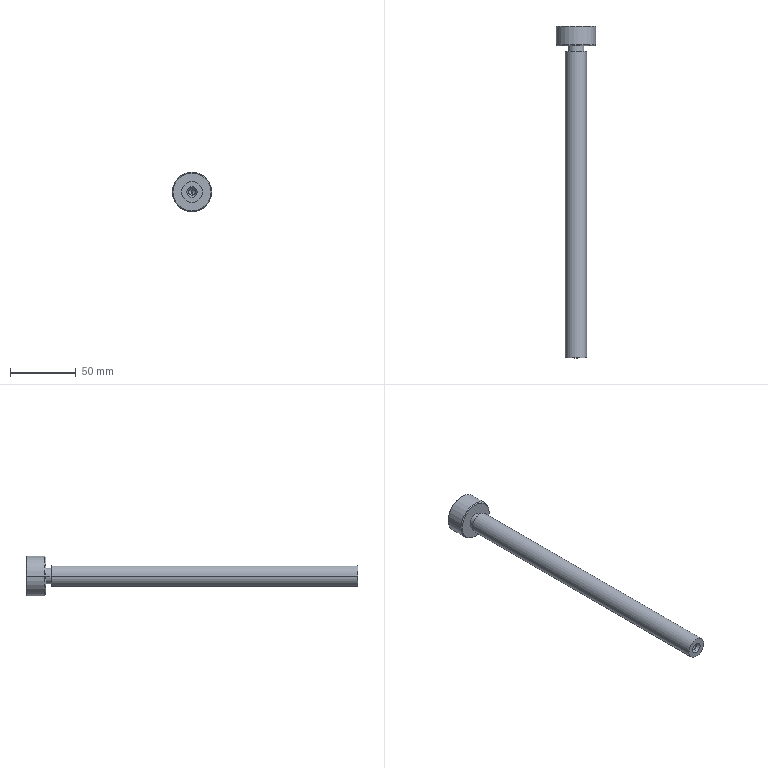Part | SolidWorks | features Chamfer 3, HoleWzd 2, Revolution 1 | 1 solid | 28 faces | box 30 x 252 x 30 mm | volume 57567 mm3 | cone 14 | cylinder 10 | plane 4 | commonest cylinder face diameters 5 x4 12 x2 16 x2 30 x2
STEP:
#1=CARTESIAN_POINT('',(0.,249.504,-2.5));
#2=VERTEX_POINT('',#1);
#3=CARTESIAN_POINT('',(0.,249.504,2.5));
#4=VERTEX_POINT('',#3);
#5=CARTESIAN_POINT('',(0.,249.504,0.));
#6=DIRECTION('',(0.,1.,0.));
#7=DIRECTION('',(0.,0.,-1.));
#8=AXIS2_PLACEMENT_3D('',#5,#6,#7);
#9=CIRCLE('',#8,2.5);
#10=EDGE_CURVE('',#2,#4,#9,.T.);
#11=ORIENTED_EDGE('',*,*,#10,.F.);
#12=CARTESIAN_POINT('',(0.,252.,-4.));
#13=VERTEX_POINT('',#12);
#14=CARTESIAN_POINT('',(0.,249.504,-2.5));
#15=DIRECTION('',(0.,0.8572,-0.515));
#16=VECTOR('',#15,1000.);
#17=LINE('',#14,#16);
#18=EDGE_CURVE('',#2,#13,#17,.T.);
#19=ORIENTED_EDGE('',*,*,#18,.T.);
#20=CARTESIAN_POINT('',(0.,252.,4.));
#21=VERTEX_POINT('',#20);
#22=CARTESIAN_POINT('',(0.,252.,0.));
#23=DIRECTION('',(0.,-1.,0.));
#24=DIRECTION('',(1.,0.,0.));
#25=AXIS2_PLACEMENT_3D('',#22,#23,#24);
#26=CIRCLE('',#25,4.);
#27=EDGE_CURVE('',#21,#13,#26,.T.);
#28=ORIENTED_EDGE('',*,*,#27,.F.);
#29=CARTESIAN_POINT('',(0.,249.504,2.5));
#30=DIRECTION('',(0.,0.8572,0.515));
#31=VECTOR('',#30,1000.);
#32=LINE('',#29,#31);
#33=EDGE_CURVE('',#4,#21,#32,.T.);
#34=ORIENTED_EDGE('',*,*,#33,.F.);
#35=EDGE_LOOP('',(#11,#19,#28,#34));
#36=FACE_OUTER_BOUND('',#35,.T.);
#37=CARTESIAN_POINT('',(0.,249.504,0.));
#38=DIRECTION('',(0.,1.,0.));
#39=DIRECTION('',(0.,0.,1.));
#40=AXIS2_PLACEMENT_3D('',#37,#38,#39);
#41=CONICAL_SURFACE('',#40,2.5,0.5411);
#42=ADVANCED_FACE('',(#36),#41,.F.);
#43=CARTESIAN_POINT('',(0.,247.,-2.5));
#44=VERTEX_POINT('',#43);
#45=CARTESIAN_POINT('',(0.,247.,2.5));
#46=VERTEX_POINT('',#45);
#47=CARTESIAN_POINT('',(0.,247.,0.));
#48=DIRECTION('',(0.,1.,0.));
#49=DIRECTION('',(0.,0.,1.));
#50=AXIS2_PLACEMENT_3D('',#47,#48,#49);
#51=CIRCLE('',#50,2.5);
#52=EDGE_CURVE('',#44,#46,#51,.T.);
#53=ORIENTED_EDGE('',*,*,#52,.F.);
#54=CARTESIAN_POINT('',(0.,252.,-2.5));
#55=DIRECTION('',(0.,1.,0.));
#56=VECTOR('',#55,1000.);
#57=LINE('',#54,#56);
#58=EDGE_CURVE('',#44,#2,#57,.T.);
#59=ORIENTED_EDGE('',*,*,#58,.T.);
#60=ORIENTED_EDGE('',*,*,#10,.T.);
#61=CARTESIAN_POINT('',(0.,252.,2.5));
#62=DIRECTION('',(0.,1.,0.));
#63=VECTOR('',#62,1000.);
#64=LINE('',#61,#63);
#65=EDGE_CURVE('',#46,#4,#64,.T.);
#66=ORIENTED_EDGE('',*,*,#65,.F.);
#67=EDGE_LOOP('',(#53,#59,#60,#66));
#68=FACE_OUTER_BOUND('',#67,.T.);
#69=CARTESIAN_POINT('',(0.,252.,0.));
#70=DIRECTION('',(0.,1.,0.));
#71=DIRECTION('',(0.,0.,1.));
#72=AXIS2_PLACEMENT_3D('',#69,#70,#71);
#73=CYLINDRICAL_SURFACE('',#72,2.5);
#74=ADVANCED_FACE('',(#68),#73,.F.);
#75=CARTESIAN_POINT('',(0.,245.498,0.));
#76=VERTEX_POINT('',#75);
#77=CARTESIAN_POINT('',(0.,247.,2.5));
#78=DIRECTION('',(0.,0.515,0.8572));
#79=VECTOR('',#78,1000.);
#80=LINE('',#77,#79);
#81=EDGE_CURVE('',#76,#46,#80,.T.);
#82=ORIENTED_EDGE('',*,*,#81,.F.);
#83=CARTESIAN_POINT('',(0.,247.,-2.5));
#84=DIRECTION('',(0.,0.515,-0.8572));
#85=VECTOR('',#84,1000.);
#86=LINE('',#83,#85);
#87=EDGE_CURVE('',#76,#44,#86,.T.);
#88=ORIENTED_EDGE('',*,*,#87,.T.);
#89=ORIENTED_EDGE('',*,*,#52,.T.);
#90=EDGE_LOOP('',(#82,#88,#89));
#91=FACE_OUTER_BOUND('',#90,.T.);
#92=CARTESIAN_POINT('',(0.,247.,0.));
#93=DIRECTION('',(0.,1.,0.));
#94=DIRECTION('',(0.,0.,1.));
#95=AXIS2_PLACEMENT_3D('',#92,#93,#94);
#96=CONICAL_SURFACE('',#95,2.5,1.03);
#97=ADVANCED_FACE('',(#91),#96,.F.);
#98=CARTESIAN_POINT('',(-14.168,252.,0.));
#99=VERTEX_POINT('',#98);
#100=CARTESIAN_POINT('',(14.168,252.,0.));
#101=VERTEX_POINT('',#100);
#102=CARTESIAN_POINT('',(0.,252.,0.));
#103=DIRECTION('',(0.,1.,0.));
#104=DIRECTION('',(1.,0.,0.));
#105=AXIS2_PLACEMENT_3D('',#102,#103,#104);
#106=CIRCLE('',#105,14.168);
#107=EDGE_CURVE('',#99,#101,#106,.T.);
#108=ORIENTED_EDGE('',*,*,#107,.F.);
#109=CARTESIAN_POINT('',(-15.,251.5,0.));
#110=VERTEX_POINT('',#109);
#111=CARTESIAN_POINT('',(-14.168,252.,0.));
#112=DIRECTION('',(-0.8572,-0.515,0.));
#113=VECTOR('',#112,1000.);
#114=LINE('',#111,#113);
#115=EDGE_CURVE('',#99,#110,#114,.T.);
#116=ORIENTED_EDGE('',*,*,#115,.T.);
#117=CARTESIAN_POINT('',(15.,251.5,0.));
#118=VERTEX_POINT('',#117);
#119=CARTESIAN_POINT('',(0.,251.5,0.));
#120=DIRECTION('',(0.,-1.,0.));
#121=DIRECTION('',(1.,0.,0.));
#122=AXIS2_PLACEMENT_3D('',#119,#120,#121);
#123=CIRCLE('',#122,15.);
#124=EDGE_CURVE('',#118,#110,#123,.T.);
#125=ORIENTED_EDGE('',*,*,#124,.F.);
#126=CARTESIAN_POINT('',(14.168,252.,0.));
#127=DIRECTION('',(0.8572,-0.515,0.));
#128=VECTOR('',#127,1000.);
#129=LINE('',#126,#128);
#130=EDGE_CURVE('',#101,#118,#129,.T.);
#131=ORIENTED_EDGE('',*,*,#130,.F.);
#132=EDGE_LOOP('',(#108,#116,#125,#131));
#133=FACE_OUTER_BOUND('',#132,.T.);
#134=CARTESIAN_POINT('',(0.,252.,0.));
#135=DIRECTION('',(0.,-1.,0.));
#136=DIRECTION('',(1.,0.,0.));
#137=AXIS2_PLACEMENT_3D('',#134,#135,#136);
#138=CONICAL_SURFACE('',#137,14.168,1.03);
#139=ADVANCED_FACE('',(#133),#138,.T.);
#140=CARTESIAN_POINT('',(14.5,237.,0.));
#141=VERTEX_POINT('',#140);
#142=CARTESIAN_POINT('',(-14.5,237.,0.));
#143=VERTEX_POINT('',#142);
#144=CARTESIAN_POINT('',(0.,237.,0.));
#145=DIRECTION('',(0.,-1.,0.));
#146=DIRECTION('',(-1.,0.,0.));
#147=AXIS2_PLACEMENT_3D('',#144,#145,#146);
#148=CIRCLE('',#147,14.5);
#149=EDGE_CURVE('',#141,#143,#148,.T.);
#150=ORIENTED_EDGE('',*,*,#149,.F.);
#151=CARTESIAN_POINT('',(15.,237.832,0.));
#152=VERTEX_POINT('',#151);
#153=CARTESIAN_POINT('',(15.,237.832,0.));
#154=DIRECTION('',(0.515,0.8572,0.));
#155=VECTOR('',#154,1000.);
#156=LINE('',#153,#155);
#157=EDGE_CURVE('',#141,#152,#156,.T.);
#158=ORIENTED_EDGE('',*,*,#157,.T.);
#159=CARTESIAN_POINT('',(-15.,237.832,0.));
#160=VERTEX_POINT('',#159);
#161=CARTESIAN_POINT('',(0.,237.832,0.));
#162=DIRECTION('',(0.,1.,0.));
#163=DIRECTION('',(-1.,0.,0.));
#164=AXIS2_PLACEMENT_3D('',#161,#162,#163);
#165=CIRCLE('',#164,15.);
#166=EDGE_CURVE('',#160,#152,#165,.T.);
#167=ORIENTED_EDGE('',*,*,#166,.F.);
#168=CARTESIAN_POINT('',(-15.,237.832,0.));
#169=DIRECTION('',(-0.515,0.8572,0.));
#170=VECTOR('',#169,1000.);
#171=LINE('',#168,#170);
#172=EDGE_CURVE('',#143,#160,#171,.T.);
#173=ORIENTED_EDGE('',*,*,#172,.F.);
#174=EDGE_LOOP('',(#150,#158,#167,#173));
#175=FACE_OUTER_BOUND('',#174,.T.);
#176=CARTESIAN_POINT('',(0.,237.832,0.));
#177=DIRECTION('',(0.,1.,0.));
#178=DIRECTION('',(-1.,0.,0.));
#179=AXIS2_PLACEMENT_3D('',#176,#177,#178);
#180=CONICAL_SURFACE('',#179,15.,0.5411);
#181=ADVANCED_FACE('',(#175),#180,.T.);
#182=CARTESIAN_POINT('',(-7.168,233.,0.));
#183=VERTEX_POINT('',#182);
#184=CARTESIAN_POINT('',(7.168,233.,0.));
#185=VERTEX_POINT('',#184);
#186=CARTESIAN_POINT('',(0.,233.,0.));
#187=DIRECTION('',(0.,1.,0.));
#188=DIRECTION('',(1.,0.,0.));
#189=AXIS2_PLACEMENT_3D('',#186,#187,#188);
#190=CIRCLE('',#189,7.168);
#191=EDGE_CURVE('',#183,#185,#190,.T.);
#192=ORIENTED_EDGE('',*,*,#191,.F.);
#193=CARTESIAN_POINT('',(-8.,232.5,0.));
#194=VERTEX_POINT('',#193);
#195=CARTESIAN_POINT('',(-7.168,233.,0.));
#196=DIRECTION('',(-0.8572,-0.515,0.));
#197=VECTOR('',#196,1000.);
#198=LINE('',#195,#197);
#199=EDGE_CURVE('',#183,#194,#198,.T.);
#200=ORIENTED_EDGE('',*,*,#199,.T.);
#201=CARTESIAN_POINT('',(8.,232.5,0.));
#202=VERTEX_POINT('',#201);
#203=CARTESIAN_POINT('',(0.,232.5,0.));
#204=DIRECTION('',(0.,-1.,0.));
#205=DIRECTION('',(1.,0.,0.));
#206=AXIS2_PLACEMENT_3D('',#203,#204,#205);
#207=CIRCLE('',#206,8.);
#208=EDGE_CURVE('',#202,#194,#207,.T.);
#209=ORIENTED_EDGE('',*,*,#208,.F.);
#210=CARTESIAN_POINT('',(7.168,233.,0.));
#211=DIRECTION('',(0.8572,-0.515,0.));
#212=VECTOR('',#211,1000.);
#213=LINE('',#210,#212);
#214=EDGE_CURVE('',#185,#202,#213,.T.);
#215=ORIENTED_EDGE('',*,*,#214,.F.);
#216=EDGE_LOOP('',(#192,#200,#209,#215));
#217=FACE_OUTER_BOUND('',#216,.T.);
#218=CARTESIAN_POINT('',(0.,233.,0.));
#219=DIRECTION('',(0.,-1.,0.));
#220=DIRECTION('',(1.,0.,0.));
#221=AXIS2_PLACEMENT_3D('',#218,#219,#220);
#222=CONICAL_SURFACE('',#221,7.168,1.03);
#223=ADVANCED_FACE('',(#217),#222,.T.);
#224=CARTESIAN_POINT('',(0.,2.496,2.5));
#225=VERTEX_POINT('',#224);
#226=CARTESIAN_POINT('',(0.,2.496,-2.5));
#227=VERTEX_POINT('',#226);
#228=CARTESIAN_POINT('',(0.,2.496,0.));
#229=DIRECTION('',(0.,-1.,0.));
#230=DIRECTION('',(0.,0.,1.));
#231=AXIS2_PLACEMENT_3D('',#228,#229,#230);
#232=CIRCLE('',#231,2.5);
#233=EDGE_CURVE('',#225,#227,#232,.T.);
#234=ORIENTED_EDGE('',*,*,#233,.F.);
#235=CARTESIAN_POINT('',(0.,0.,4.));
#236=VERTEX_POINT('',#235);
#237=CARTESIAN_POINT('',(0.,2.496,2.5));
#238=DIRECTION('',(0.,-0.8572,0.515));
#239=VECTOR('',#238,1000.);
#240=LINE('',#237,#239);
#241=EDGE_CURVE('',#225,#236,#240,.T.);
#242=ORIENTED_EDGE('',*,*,#241,.T.);
#243=CARTESIAN_POINT('',(0.,0.,-4.));
#244=VERTEX_POINT('',#243);
#245=CARTESIAN_POINT('',(0.,0.,0.));
#246=DIRECTION('',(0.,1.,0.));
#247=DIRECTION('',(-1.,0.,0.));
#248=AXIS2_PLACEMENT_3D('',#245,#246,#247);
#249=CIRCLE('',#248,4.);
#250=EDGE_CURVE('',#244,#236,#249,.T.);
#251=ORIENTED_EDGE('',*,*,#250,.F.);
#252=CARTESIAN_POINT('',(0.,2.496,-2.5));
#253=DIRECTION('',(0.,-0.8572,-0.515));
#254=VECTOR('',#253,1000.);
#255=LINE('',#252,#254);
#256=EDGE_CURVE('',#227,#244,#255,.T.);
#257=ORIENTED_EDGE('',*,*,#256,.F.);
#258=EDGE_LOOP('',(#234,#242,#251,#257));
#259=FACE_OUTER_BOUND('',#258,.T.);
#260=CARTESIAN_POINT('',(0.,2.496,0.));
#261=DIRECTION('',(0.,-1.,0.));
#262=DIRECTION('',(0.,0.,-1.));
#263=AXIS2_PLACEMENT_3D('',#260,#261,#262);
#264=CONICAL_SURFACE('',#263,2.5,0.5411);
#265=ADVANCED_FACE('',(#259),#264,.F.);
#266=CARTESIAN_POINT('',(0.,5.,2.5));
#267=VERTEX_POINT('',#266);
#268=CARTESIAN_POINT('',(0.,5.,-2.5));
#269=VERTEX_POINT('',#268);
#270=CARTESIAN_POINT('',(0.,5.,0.));
#271=DIRECTION('',(0.,-1.,0.));
#272=DIRECTION('',(0.,0.,-1.));
#273=AXIS2_PLACEMENT_3D('',#270,#271,#272);
#274=CIRCLE('',#273,2.5);
#275=EDGE_CURVE('',#267,#269,#274,.T.);
#276=ORIENTED_EDGE('',*,*,#275,.F.);
#277=CARTESIAN_POINT('',(0.,0.,2.5));
#278=DIRECTION('',(0.,-1.,0.));
#279=VECTOR('',#278,1000.);
#280=LINE('',#277,#279);
#281=EDGE_CURVE('',#267,#225,#280,.T.);
#282=ORIENTED_EDGE('',*,*,#281,.T.);
#283=ORIENTED_EDGE('',*,*,#233,.T.);
#284=CARTESIAN_POINT('',(0.,0.,-2.5));
#285=DIRECTION('',(0.,-1.,0.));
#286=VECTOR('',#285,1000.);
#287=LINE('',#284,#286);
#288=EDGE_CURVE('',#269,#227,#287,.T.);
#289=ORIENTED_EDGE('',*,*,#288,.F.);
#290=EDGE_LOOP('',(#276,#282,#283,#289));
#291=FACE_OUTER_BOUND('',#290,.T.);
#292=CARTESIAN_POINT('',(0.,0.,0.));
#293=DIRECTION('',(0.,-1.,0.));
#294=DIRECTION('',(0.,0.,-1.));
#295=AXIS2_PLACEMENT_3D('',#292,#293,#294);
#296=CYLINDRICAL_SURFACE('',#295,2.5);
#297=ADVANCED_FACE('',(#291),#296,.F.);
#298=CARTESIAN_POINT('',(0.,6.502,0.));
#299=VERTEX_POINT('',#298);
#300=CARTESIAN_POINT('',(0.,5.,-2.5));
#301=DIRECTION('',(0.,-0.515,-0.8572));
#302=VECTOR('',#301,1000.);
#303=LINE('',#300,#302);
#304=EDGE_CURVE('',#299,#269,#303,.T.);
#305=ORIENTED_EDGE('',*,*,#304,.F.);
#306=CARTESIAN_POINT('',(0.,5.,2.5));
#307=DIRECTION('',(0.,-0.515,0.8572));
#308=VECTOR('',#307,1000.);
#309=LINE('',#306,#308);
#310=EDGE_CURVE('',#299,#267,#309,.T.);
#311=ORIENTED_EDGE('',*,*,#310,.T.);
#312=ORIENTED_EDGE('',*,*,#275,.T.);
#313=EDGE_LOOP('',(#305,#311,#312));
#314=FACE_OUTER_BOUND('',#313,.T.);
#315=CARTESIAN_POINT('',(0.,5.,0.));
#316=DIRECTION('',(0.,-1.,0.));
#317=DIRECTION('',(0.,0.,-1.));
#318=AXIS2_PLACEMENT_3D('',#315,#316,#317);
#319=CONICAL_SURFACE('',#318,2.5,1.03);
#320=ADVANCED_FACE('',(#314),#319,.F.);
#321=ORIENTED_EDGE('',*,*,#166,.T.);
#322=CARTESIAN_POINT('',(15.,252.,0.));
#323=DIRECTION('',(0.,1.,0.));
#324=VECTOR('',#323,1000.);
#325=LINE('',#322,#324);
#326=EDGE_CURVE('',#152,#118,#325,.T.);
#327=ORIENTED_EDGE('',*,*,#326,.T.);
#328=ORIENTED_EDGE('',*,*,#124,.T.);
#329=CARTESIAN_POINT('',(-15.,252.,0.));
#330=DIRECTION('',(0.,1.,0.));
#331=VECTOR('',#330,1000.);
#332=LINE('',#329,#331);
#333=EDGE_CURVE('',#160,#110,#332,.T.);
#334=ORIENTED_EDGE('',*,*,#333,.F.);
#335=EDGE_LOOP('',(#321,#327,#328,#334));
#336=FACE_OUTER_BOUND('',#335,.T.);
#337=CARTESIAN_POINT('',(0.,252.,0.));
#338=DIRECTION('',(0.,1.,0.));
#339=DIRECTION('',(-1.,0.,0.));
#340=AXIS2_PLACEMENT_3D('',#337,#338,#339);
#341=CYLINDRICAL_SURFACE('',#340,15.);
#342=ADVANCED_FACE('',(#336),#341,.T.);
#343=CARTESIAN_POINT('',(-8.,0.,0.));
#344=VERTEX_POINT('',#343);
#345=CARTESIAN_POINT('',(8.,0.,0.));
#346=VERTEX_POINT('',#345);
#347=CARTESIAN_POINT('',(0.,0.,0.));
#348=DIRECTION('',(0.,1.,0.));
#349=DIRECTION('',(-1.,0.,0.));
#350=AXIS2_PLACEMENT_3D('',#347,#348,#349);
#351=CIRCLE('',#350,8.);
#352=EDGE_CURVE('',#344,#346,#351,.T.);
#353=ORIENTED_EDGE('',*,*,#352,.T.);
#354=CARTESIAN_POINT('',(8.,252.,0.));
#355=DIRECTION('',(0.,1.,0.));
#356=VECTOR('',#355,1000.);
#357=LINE('',#354,#356);
#358=EDGE_CURVE('',#346,#202,#357,.T.);
#359=ORIENTED_EDGE('',*,*,#358,.T.);
#360=ORIENTED_EDGE('',*,*,#208,.T.);
#361=CARTESIAN_POINT('',(-8.,252.,0.));
#362=DIRECTION('',(0.,1.,0.));
#363=VECTOR('',#362,1000.);
#364=LINE('',#361,#363);
#365=EDGE_CURVE('',#344,#194,#364,.T.);
#366=ORIENTED_EDGE('',*,*,#365,.F.);
#367=EDGE_LOOP('',(#353,#359,#360,#366));
#368=FACE_OUTER_BOUND('',#367,.T.);
#369=CARTESIAN_POINT('',(0.,252.,0.));
#370=DIRECTION('',(0.,1.,0.));
#371=DIRECTION('',(-1.,0.,0.));
#372=AXIS2_PLACEMENT_3D('',#369,#370,#371);
#373=CYLINDRICAL_SURFACE('',#372,8.);
#374=ADVANCED_FACE('',(#368),#373,.T.);
#375=CARTESIAN_POINT('',(-6.,233.,0.));
#376=VERTEX_POINT('',#375);
#377=CARTESIAN_POINT('',(6.,233.,0.));
#378=VERTEX_POINT('',#377);
#379=CARTESIAN_POINT('',(0.,233.,0.));
#380=DIRECTION('',(0.,1.,0.));
#381=DIRECTION('',(-1.,0.,0.));
#382=AXIS2_PLACEMENT_3D('',#379,#380,#381);
#383=CIRCLE('',#382,6.);
#384=EDGE_CURVE('',#376,#378,#383,.T.);
#385=ORIENTED_EDGE('',*,*,#384,.T.);
#386=CARTESIAN_POINT('',(6.,237.,0.));
#387=VERTEX_POINT('',#386);
#388=CARTESIAN_POINT('',(6.,252.,0.));
#389=DIRECTION('',(0.,1.,0.));
#390=VECTOR('',#389,1000.);
#391=LINE('',#388,#390);
#392=EDGE_CURVE('',#378,#387,#391,.T.);
#393=ORIENTED_EDGE('',*,*,#392,.T.);
#394=CARTESIAN_POINT('',(-6.,237.,0.));
#395=VERTEX_POINT('',#394);
#396=CARTESIAN_POINT('',(0.,237.,0.));
#397=DIRECTION('',(0.,1.,0.));
#398=DIRECTION('',(-1.,0.,0.));
#399=AXIS2_PLACEMENT_3D('',#396,#397,#398);
#400=CIRCLE('',#399,6.);
#401=EDGE_CURVE('',#395,#387,#400,.T.);
#402=ORIENTED_EDGE('',*,*,#401,.F.);
#403=CARTESIAN_POINT('',(-6.,252.,0.));
#404=DIRECTION('',(0.,1.,0.));
#405=VECTOR('',#404,1000.);
#406=LINE('',#403,#405);
#407=EDGE_CURVE('',#376,#395,#406,.T.);
#408=ORIENTED_EDGE('',*,*,#407,.F.);
#409=EDGE_LOOP('',(#385,#393,#402,#408));
#410=FACE_OUTER_BOUND('',#409,.T.);
#411=CARTESIAN_POINT('',(0.,252.,0.));
#412=DIRECTION('',(0.,1.,0.));
#413=DIRECTION('',(-1.,0.,0.));
#414=AXIS2_PLACEMENT_3D('',#411,#412,#413);
#415=CYLINDRICAL_SURFACE('',#414,6.);
#416=ADVANCED_FACE('',(#410),#415,.T.);
#417=ORIENTED_EDGE('',*,*,#392,.F.);
#418=CARTESIAN_POINT('',(0.,233.,0.));
#419=DIRECTION('',(0.,1.,0.));
#420=DIRECTION('',(-1.,0.,0.));
#421=AXIS2_PLACEMENT_3D('',#418,#419,#420);
#422=CIRCLE('',#421,6.);
#423=EDGE_CURVE('',#378,#376,#422,.T.);
#424=ORIENTED_EDGE('',*,*,#423,.T.);
#425=ORIENTED_EDGE('',*,*,#407,.T.);
#426=CARTESIAN_POINT('',(0.,237.,0.));
#427=DIRECTION('',(0.,1.,0.));
#428=DIRECTION('',(-1.,0.,0.));
#429=AXIS2_PLACEMENT_3D('',#426,#427,#428);
#430=CIRCLE('',#429,6.);
#431=EDGE_CURVE('',#387,#395,#430,.T.);
#432=ORIENTED_EDGE('',*,*,#431,.F.);
#433=EDGE_LOOP('',(#417,#424,#425,#432));
#434=FACE_OUTER_BOUND('',#433,.T.);
#435=CARTESIAN_POINT('',(0.,252.,0.));
#436=DIRECTION('',(0.,1.,0.));
#437=DIRECTION('',(-1.,0.,0.));
#438=AXIS2_PLACEMENT_3D('',#435,#436,#437);
#439=CYLINDRICAL_SURFACE('',#438,6.);
#440=ADVANCED_FACE('',(#434),#439,.T.);
#441=CARTESIAN_POINT('',(0.,233.,0.));
#442=DIRECTION('',(0.,1.,0.));
#443=DIRECTION('',(1.,0.,0.));
#444=AXIS2_PLACEMENT_3D('',#441,#442,#443);
#445=CIRCLE('',#444,7.168);
#446=EDGE_CURVE('',#185,#183,#445,.T.);
#447=ORIENTED_EDGE('',*,*,#446,.T.);
#448=ORIENTED_EDGE('',*,*,#191,.T.);
#449=EDGE_LOOP('',(#447,#448));
#450=FACE_OUTER_BOUND('',#449,.T.);
#451=ORIENTED_EDGE('',*,*,#384,.F.);
#452=ORIENTED_EDGE('',*,*,#423,.F.);
#453=EDGE_LOOP('',(#451,#452));
#454=FACE_BOUND('',#453,.T.);
#455=CARTESIAN_POINT('',(8.,233.,0.));
#456=DIRECTION('',(0.,-1.,0.));
#457=DIRECTION('',(1.,0.,0.));
#458=AXIS2_PLACEMENT_3D('',#455,#456,#457);
#459=PLANE('',#458);
#460=ADVANCED_FACE('',(#450,#454),#459,.F.);
#461=ORIENTED_EDGE('',*,*,#358,.F.);
#462=CARTESIAN_POINT('',(0.,0.,0.));
#463=DIRECTION('',(0.,1.,0.));
#464=DIRECTION('',(-1.,0.,0.));
#465=AXIS2_PLACEMENT_3D('',#462,#463,#464);
#466=CIRCLE('',#465,8.);
#467=EDGE_CURVE('',#346,#344,#466,.T.);
#468=ORIENTED_EDGE('',*,*,#467,.T.);
#469=ORIENTED_EDGE('',*,*,#365,.T.);
#470=CARTESIAN_POINT('',(0.,232.5,0.));
#471=DIRECTION('',(0.,-1.,0.));
#472=DIRECTION('',(1.,0.,0.));
#473=AXIS2_PLACEMENT_3D('',#470,#471,#472);
#474=CIRCLE('',#473,8.);
#475=EDGE_CURVE('',#194,#202,#474,.T.);
#476=ORIENTED_EDGE('',*,*,#475,.T.);
#477=EDGE_LOOP('',(#461,#468,#469,#476));
#478=FACE_OUTER_BOUND('',#477,.T.);
#479=CARTESIAN_POINT('',(0.,252.,0.));
#480=DIRECTION('',(0.,1.,0.));
#481=DIRECTION('',(-1.,0.,0.));
#482=AXIS2_PLACEMENT_3D('',#479,#480,#481);
#483=CYLINDRICAL_SURFACE('',#482,8.);
#484=ADVANCED_FACE('',(#478),#483,.T.);
#485=ORIENTED_EDGE('',*,*,#250,.T.);
#486=CARTESIAN_POINT('',(0.,0.,0.));
#487=DIRECTION('',(0.,1.,0.));
#488=DIRECTION('',(-1.,0.,0.));
#489=AXIS2_PLACEMENT_3D('',#486,#487,#488);
#490=CIRCLE('',#489,4.);
#491=EDGE_CURVE('',#236,#244,#490,.T.);
#492=ORIENTED_EDGE('',*,*,#491,.T.);
#493=EDGE_LOOP('',(#485,#492));
#494=FACE_BOUND('',#493,.T.);
#495=ORIENTED_EDGE('',*,*,#352,.F.);
#496=ORIENTED_EDGE('',*,*,#467,.F.);
#497=EDGE_LOOP('',(#495,#496));
#498=FACE_OUTER_BOUND('',#497,.T.);
#499=CARTESIAN_POINT('',(0.,0.,0.));
#500=DIRECTION('',(0.,1.,0.));
#501=DIRECTION('',(-1.,0.,0.));
#502=AXIS2_PLACEMENT_3D('',#499,#500,#501);
#503=PLANE('',#502);
#504=ADVANCED_FACE('',(#494,#498),#503,.F.);
#505=ORIENTED_EDGE('',*,*,#27,.T.);
#506=CARTESIAN_POINT('',(0.,252.,0.));
#507=DIRECTION('',(0.,-1.,0.));
#508=DIRECTION('',(1.,0.,0.));
#509=AXIS2_PLACEMENT_3D('',#506,#507,#508);
#510=CIRCLE('',#509,4.);
#511=EDGE_CURVE('',#13,#21,#510,.T.);
#512=ORIENTED_EDGE('',*,*,#511,.T.);
#513=EDGE_LOOP('',(#505,#512));
#514=FACE_BOUND('',#513,.T.);
#515=CARTESIAN_POINT('',(0.,252.,0.));
#516=DIRECTION('',(0.,1.,0.));
#517=DIRECTION('',(1.,0.,0.));
#518=AXIS2_PLACEMENT_3D('',#515,#516,#517);
#519=CIRCLE('',#518,14.168);
#520=EDGE_CURVE('',#101,#99,#519,.T.);
#521=ORIENTED_EDGE('',*,*,#520,.T.);
#522=ORIENTED_EDGE('',*,*,#107,.T.);
#523=EDGE_LOOP('',(#521,#522));
#524=FACE_OUTER_BOUND('',#523,.T.);
#525=CARTESIAN_POINT('',(0.,252.,0.));
#526=DIRECTION('',(0.,-1.,0.));
#527=DIRECTION('',(1.,0.,0.));
#528=AXIS2_PLACEMENT_3D('',#525,#526,#527);
#529=PLANE('',#528);
#530=ADVANCED_FACE('',(#514,#524),#529,.F.);
#531=ORIENTED_EDGE('',*,*,#326,.F.);
#532=CARTESIAN_POINT('',(0.,237.832,0.));
#533=DIRECTION('',(0.,1.,0.));
#534=DIRECTION('',(-1.,0.,0.));
#535=AXIS2_PLACEMENT_3D('',#532,#533,#534);
#536=CIRCLE('',#535,15.);
#537=EDGE_CURVE('',#152,#160,#536,.T.);
#538=ORIENTED_EDGE('',*,*,#537,.T.);
#539=ORIENTED_EDGE('',*,*,#333,.T.);
#540=CARTESIAN_POINT('',(0.,251.5,0.));
#541=DIRECTION('',(0.,-1.,0.));
#542=DIRECTION('',(1.,0.,0.));
#543=AXIS2_PLACEMENT_3D('',#540,#541,#542);
#544=CIRCLE('',#543,15.);
#545=EDGE_CURVE('',#110,#118,#544,.T.);
#546=ORIENTED_EDGE('',*,*,#545,.T.);
#547=EDGE_LOOP('',(#531,#538,#539,#546));
#548=FACE_OUTER_BOUND('',#547,.T.);
#549=CARTESIAN_POINT('',(0.,252.,0.));
#550=DIRECTION('',(0.,1.,0.));
#551=DIRECTION('',(-1.,0.,0.));
#552=AXIS2_PLACEMENT_3D('',#549,#550,#551);
#553=CYLINDRICAL_SURFACE('',#552,15.);
#554=ADVANCED_FACE('',(#548),#553,.T.);
#555=CARTESIAN_POINT('',(0.,237.,0.));
#556=DIRECTION('',(0.,-1.,0.));
#557=DIRECTION('',(-1.,0.,0.));
#558=AXIS2_PLACEMENT_3D('',#555,#556,#557);
#559=CIRCLE('',#558,14.5);
#560=EDGE_CURVE('',#143,#141,#559,.T.);
#561=ORIENTED_EDGE('',*,*,#560,.T.);
#562=ORIENTED_EDGE('',*,*,#149,.T.);
#563=EDGE_LOOP('',(#561,#562));
#564=FACE_OUTER_BOUND('',#563,.T.);
#565=ORIENTED_EDGE('',*,*,#401,.T.);
#566=ORIENTED_EDGE('',*,*,#431,.T.);
#567=EDGE_LOOP('',(#565,#566));
#568=FACE_BOUND('',#567,.T.);
#569=CARTESIAN_POINT('',(15.,237.,0.));
#570=DIRECTION('',(0.,1.,0.));
#571=DIRECTION('',(-1.,0.,0.));
#572=AXIS2_PLACEMENT_3D('',#569,#570,#571);
#573=PLANE('',#572);
#574=ADVANCED_FACE('',(#564,#568),#573,.F.);
#575=ORIENTED_EDGE('',*,*,#310,.F.);
#576=ORIENTED_EDGE('',*,*,#304,.T.);
#577=CARTESIAN_POINT('',(0.,5.,0.));
#578=DIRECTION('',(0.,-1.,0.));
#579=DIRECTION('',(0.,0.,-1.));
#580=AXIS2_PLACEMENT_3D('',#577,#578,#579);
#581=CIRCLE('',#580,2.5);
#582=EDGE_CURVE('',#269,#267,#581,.T.);
#583=ORIENTED_EDGE('',*,*,#582,.T.);
#584=EDGE_LOOP('',(#575,#576,#583));
#585=FACE_OUTER_BOUND('',#584,.T.);
#586=CARTESIAN_POINT('',(0.,5.,0.));
#587=DIRECTION('',(0.,-1.,0.));
#588=DIRECTION('',(0.,0.,-1.));
#589=AXIS2_PLACEMENT_3D('',#586,#587,#588);
#590=CONICAL_SURFACE('',#589,2.5,1.03);
#591=ADVANCED_FACE('',(#585),#590,.F.);
#592=ORIENTED_EDGE('',*,*,#281,.F.);
#593=ORIENTED_EDGE('',*,*,#582,.F.);
#594=ORIENTED_EDGE('',*,*,#288,.T.);
#595=CARTESIAN_POINT('',(0.,2.496,0.));
#596=DIRECTION('',(0.,-1.,0.));
#597=DIRECTION('',(0.,0.,1.));
#598=AXIS2_PLACEMENT_3D('',#595,#596,#597);
#599=CIRCLE('',#598,2.5);
#600=EDGE_CURVE('',#227,#225,#599,.T.);
#601=ORIENTED_EDGE('',*,*,#600,.T.);
#602=EDGE_LOOP('',(#592,#593,#594,#601));
#603=FACE_OUTER_BOUND('',#602,.T.);
#604=CARTESIAN_POINT('',(0.,0.,0.));
#605=DIRECTION('',(0.,-1.,0.));
#606=DIRECTION('',(0.,0.,-1.));
#607=AXIS2_PLACEMENT_3D('',#604,#605,#606);
#608=CYLINDRICAL_SURFACE('',#607,2.5);
#609=ADVANCED_FACE('',(#603),#608,.F.);
#610=ORIENTED_EDGE('',*,*,#241,.F.);
#611=ORIENTED_EDGE('',*,*,#600,.F.);
#612=ORIENTED_EDGE('',*,*,#256,.T.);
#613=ORIENTED_EDGE('',*,*,#491,.F.);
#614=EDGE_LOOP('',(#610,#611,#612,#613));
#615=FACE_OUTER_BOUND('',#614,.T.);
#616=CARTESIAN_POINT('',(0.,2.496,0.));
#617=DIRECTION('',(0.,-1.,0.));
#618=DIRECTION('',(0.,0.,-1.));
#619=AXIS2_PLACEMENT_3D('',#616,#617,#618);
#620=CONICAL_SURFACE('',#619,2.5,0.5411);
#621=ADVANCED_FACE('',(#615),#620,.F.);
#622=ORIENTED_EDGE('',*,*,#199,.F.);
#623=ORIENTED_EDGE('',*,*,#446,.F.);
#624=ORIENTED_EDGE('',*,*,#214,.T.);
#625=ORIENTED_EDGE('',*,*,#475,.F.);
#626=EDGE_LOOP('',(#622,#623,#624,#625));
#627=FACE_OUTER_BOUND('',#626,.T.);
#628=CARTESIAN_POINT('',(0.,233.,0.));
#629=DIRECTION('',(0.,-1.,0.));
#630=DIRECTION('',(1.,0.,0.));
#631=AXIS2_PLACEMENT_3D('',#628,#629,#630);
#632=CONICAL_SURFACE('',#631,7.168,1.03);
#633=ADVANCED_FACE('',(#627),#632,.T.);
#634=ORIENTED_EDGE('',*,*,#157,.F.);
#635=ORIENTED_EDGE('',*,*,#560,.F.);
#636=ORIENTED_EDGE('',*,*,#172,.T.);
#637=ORIENTED_EDGE('',*,*,#537,.F.);
#638=EDGE_LOOP('',(#634,#635,#636,#637));
#639=FACE_OUTER_BOUND('',#638,.T.);
#640=CARTESIAN_POINT('',(0.,237.832,0.));
#641=DIRECTION('',(0.,1.,0.));
#642=DIRECTION('',(-1.,0.,0.));
#643=AXIS2_PLACEMENT_3D('',#640,#641,#642);
#644=CONICAL_SURFACE('',#643,15.,0.5411);
#645=ADVANCED_FACE('',(#639),#644,.T.);
#646=ORIENTED_EDGE('',*,*,#115,.F.);
#647=ORIENTED_EDGE('',*,*,#520,.F.);
#648=ORIENTED_EDGE('',*,*,#130,.T.);
#649=ORIENTED_EDGE('',*,*,#545,.F.);
#650=EDGE_LOOP('',(#646,#647,#648,#649));
#651=FACE_OUTER_BOUND('',#650,.T.);
#652=CARTESIAN_POINT('',(0.,252.,0.));
#653=DIRECTION('',(0.,-1.,0.));
#654=DIRECTION('',(1.,0.,0.));
#655=AXIS2_PLACEMENT_3D('',#652,#653,#654);
#656=CONICAL_SURFACE('',#655,14.168,1.03);
#657=ADVANCED_FACE('',(#651),#656,.T.);
#658=ORIENTED_EDGE('',*,*,#87,.F.);
#659=ORIENTED_EDGE('',*,*,#81,.T.);
#660=CARTESIAN_POINT('',(0.,247.,0.));
#661=DIRECTION('',(0.,1.,0.));
#662=DIRECTION('',(0.,0.,1.));
#663=AXIS2_PLACEMENT_3D('',#660,#661,#662);
#664=CIRCLE('',#663,2.5);
#665=EDGE_CURVE('',#46,#44,#664,.T.);
#666=ORIENTED_EDGE('',*,*,#665,.T.);
#667=EDGE_LOOP('',(#658,#659,#666));
#668=FACE_OUTER_BOUND('',#667,.T.);
#669=CARTESIAN_POINT('',(0.,247.,0.));
#670=DIRECTION('',(0.,1.,0.));
#671=DIRECTION('',(0.,0.,1.));
#672=AXIS2_PLACEMENT_3D('',#669,#670,#671);
#673=CONICAL_SURFACE('',#672,2.5,1.03);
#674=ADVANCED_FACE('',(#668),#673,.F.);
#675=ORIENTED_EDGE('',*,*,#58,.F.);
#676=ORIENTED_EDGE('',*,*,#665,.F.);
#677=ORIENTED_EDGE('',*,*,#65,.T.);
#678=CARTESIAN_POINT('',(0.,249.504,0.));
#679=DIRECTION('',(0.,1.,0.));
#680=DIRECTION('',(0.,0.,-1.));
#681=AXIS2_PLACEMENT_3D('',#678,#679,#680);
#682=CIRCLE('',#681,2.5);
#683=EDGE_CURVE('',#4,#2,#682,.T.);
#684=ORIENTED_EDGE('',*,*,#683,.T.);
#685=EDGE_LOOP('',(#675,#676,#677,#684));
#686=FACE_OUTER_BOUND('',#685,.T.);
#687=CARTESIAN_POINT('',(0.,252.,0.));
#688=DIRECTION('',(0.,1.,0.));
#689=DIRECTION('',(0.,0.,1.));
#690=AXIS2_PLACEMENT_3D('',#687,#688,#689);
#691=CYLINDRICAL_SURFACE('',#690,2.5);
#692=ADVANCED_FACE('',(#686),#691,.F.);
#693=ORIENTED_EDGE('',*,*,#18,.F.);
#694=ORIENTED_EDGE('',*,*,#683,.F.);
#695=ORIENTED_EDGE('',*,*,#33,.T.);
#696=ORIENTED_EDGE('',*,*,#511,.F.);
#697=EDGE_LOOP('',(#693,#694,#695,#696));
#698=FACE_OUTER_BOUND('',#697,.T.);
#699=CARTESIAN_POINT('',(0.,249.504,0.));
#700=DIRECTION('',(0.,1.,0.));
#701=DIRECTION('',(0.,0.,1.));
#702=AXIS2_PLACEMENT_3D('',#699,#700,#701);
#703=CONICAL_SURFACE('',#702,2.5,0.5411);
#704=ADVANCED_FACE('',(#698),#703,.F.);
#705=CLOSED_SHELL('',(#42,#74,#97,#139,#181,#223,#265,#297,#320,#342,#374,#416,#440,#460,#484,#504,#530,#554,#574,#591,#609,#621,#633,#645,#657,#674,#692,#704));
#706=MANIFOLD_SOLID_BREP('',#705);
#707=CARTESIAN_POINT('',(0.,0.,0.));
#708=DIRECTION('',(0.,0.,1.));
#709=DIRECTION('',(1.,0.,0.));
#710=AXIS2_PLACEMENT_3D('',#707,#708,#709);
#711=(LENGTH_UNIT()NAMED_UNIT(*)SI_UNIT(.MILLI.,.METRE.));
#712=UNCERTAINTY_MEASURE_WITH_UNIT(LENGTH_MEASURE(0.00001),#711,'','');
#713=(NAMED_UNIT(*)PLANE_ANGLE_UNIT()SI_UNIT($,.RADIAN.));
#714=(NAMED_UNIT(*)SI_UNIT($,.STERADIAN.)SOLID_ANGLE_UNIT());
#715=(GEOMETRIC_REPRESENTATION_CONTEXT(3)GLOBAL_UNCERTAINTY_ASSIGNED_CONTEXT((#712))GLOBAL_UNIT_ASSIGNED_CONTEXT((#711,#713,#714))REPRESENTATION_CONTEXT('',''));
#716=ADVANCED_BREP_SHAPE_REPRESENTATION('',(#706,#710),#715);